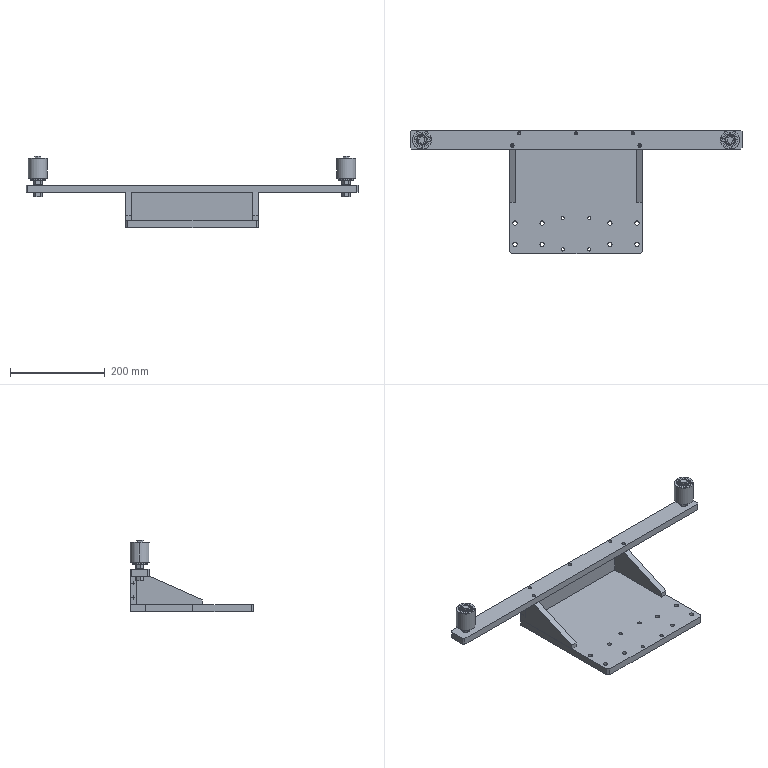Part | SolidWorks | features AEMSimFeature 1 | 21 solids | 628 faces | box 700 x 260 x 150.5 mm | volume 1942700 mm3 | cylinder 192 | torus 176 | plane 124 | sphere 96 | cone 40 | commonest cylinder face diameters 5 x32 7 x32 11 x24 9 x16 18.667 x16 25.333 x16